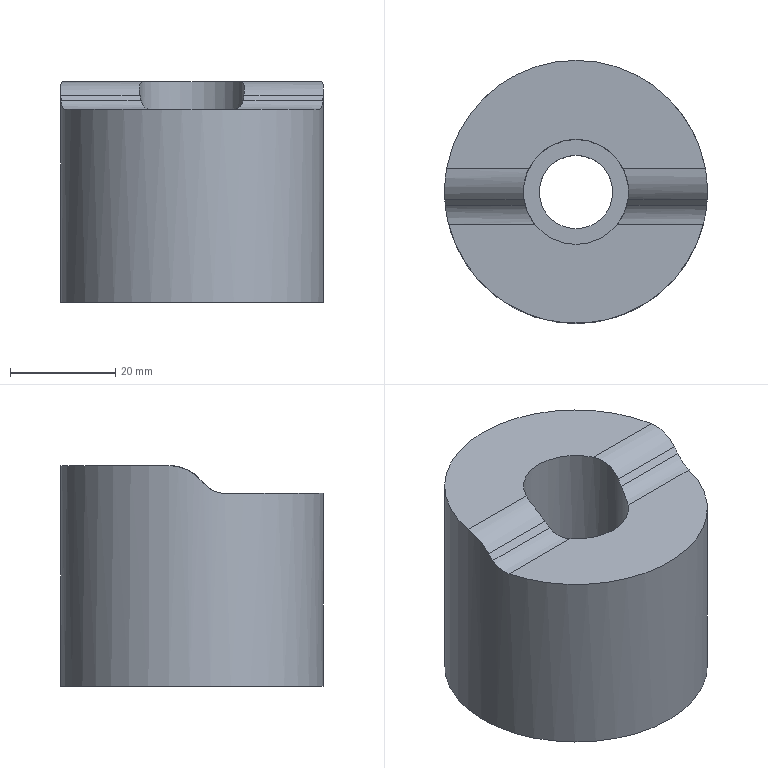Part | NX | features solid 2 | 1 solid | 13 faces | box 50 x 50 x 42.008 mm | volume 68340 mm3 | cylinder 7 | plane 6 | commonest cylinder face diameters 10 x2 16 x2 14 x1 20 x1 50 x1
STEP:
#1=CARTESIAN_POINT('',(215.,-615.,50.));
#2=VERTEX_POINT('',#1);
#3=CARTESIAN_POINT('',(215.,-590.,50.));
#4=DIRECTION('',(0.,0.,1.));
#5=DIRECTION('',(0.,-1.,0.));
#6=AXIS2_PLACEMENT_3D('',#3,#4,#5);
#7=CIRCLE('',#6,25.);
#8=EDGE_CURVE('',#2,#2,#7,.T.);
#9=ORIENTED_EDGE('',*,*,#8,.T.);
#10=EDGE_LOOP('',(#9));
#11=FACE_BOUND('',#10,.T.);
#12=CARTESIAN_POINT('',(239.954,-591.512,89.423));
#13=VERTEX_POINT('',#12);
#14=CARTESIAN_POINT('',(239.614,-585.624,92.008));
#15=VERTEX_POINT('',#14);
#16=CARTESIAN_POINT('',(239.954,-591.512,89.423));
#17=CARTESIAN_POINT('',(240.046,-590.003,91.064));
#18=CARTESIAN_POINT('',(240.005,-587.821,92.008));
#19=CARTESIAN_POINT('',(239.614,-585.624,92.008));
#20=B_SPLINE_CURVE_WITH_KNOTS('',3,(#16,#17,#18,#19),.UNSPECIFIED.,.F.,.F.,(4,4),(0.,0.006601),.UNSPECIFIED.);
#21=EDGE_CURVE('',#13,#15,#20,.T.);
#22=ORIENTED_EDGE('',*,*,#21,.F.);
#23=CARTESIAN_POINT('',(239.872,-592.524,88.323));
#24=VERTEX_POINT('',#23);
#25=CARTESIAN_POINT('',(215.,-590.,91.067));
#26=DIRECTION('',(0.,0.736,-0.677));
#27=DIRECTION('',(0.,-0.677,-0.736));
#28=AXIS2_PLACEMENT_3D('',#25,#26,#27);
#29=ELLIPSE('',#28,36.93,25.);
#30=EDGE_CURVE('',#13,#24,#29,.T.);
#31=ORIENTED_EDGE('',*,*,#30,.T.);
#32=CARTESIAN_POINT('',(239.218,-596.204,86.708));
#33=VERTEX_POINT('',#32);
#34=CARTESIAN_POINT('',(239.872,-592.524,88.323));
#35=CARTESIAN_POINT('',(239.776,-593.476,87.288));
#36=CARTESIAN_POINT('',(239.568,-594.839,86.708));
#37=CARTESIAN_POINT('',(239.218,-596.204,86.708));
#38=B_SPLINE_CURVE_WITH_KNOTS('',3,(#34,#35,#36,#37),.UNSPECIFIED.,.F.,.F.,(4,4),(0.,0.004167),.UNSPECIFIED.);
#39=EDGE_CURVE('',#24,#33,#38,.T.);
#40=ORIENTED_EDGE('',*,*,#39,.T.);
#41=CARTESIAN_POINT('',(190.782,-596.204,86.708));
#42=VERTEX_POINT('',#41);
#43=CARTESIAN_POINT('',(215.,-590.,86.708));
#44=DIRECTION('',(0.,0.,1.));
#45=DIRECTION('',(0.,-1.,0.));
#46=AXIS2_PLACEMENT_3D('',#43,#44,#45);
#47=CIRCLE('',#46,25.);
#48=EDGE_CURVE('',#42,#33,#47,.T.);
#49=ORIENTED_EDGE('',*,*,#48,.F.);
#50=CARTESIAN_POINT('',(190.128,-592.524,88.323));
#51=VERTEX_POINT('',#50);
#52=CARTESIAN_POINT('',(190.782,-596.204,86.708));
#53=CARTESIAN_POINT('',(190.432,-594.839,86.708));
#54=CARTESIAN_POINT('',(190.224,-593.476,87.288));
#55=CARTESIAN_POINT('',(190.128,-592.524,88.323));
#56=B_SPLINE_CURVE_WITH_KNOTS('',3,(#52,#53,#54,#55),.UNSPECIFIED.,.F.,.F.,(4,4),(0.,0.004169),.UNSPECIFIED.);
#57=EDGE_CURVE('',#42,#51,#56,.T.);
#58=ORIENTED_EDGE('',*,*,#57,.T.);
#59=CARTESIAN_POINT('',(190.046,-591.512,89.423));
#60=VERTEX_POINT('',#59);
#61=CARTESIAN_POINT('',(215.,-590.,91.067));
#62=DIRECTION('',(0.,0.736,-0.677));
#63=DIRECTION('',(0.,-0.677,-0.736));
#64=AXIS2_PLACEMENT_3D('',#61,#62,#63);
#65=ELLIPSE('',#64,36.93,25.);
#66=EDGE_CURVE('',#51,#60,#65,.T.);
#67=ORIENTED_EDGE('',*,*,#66,.T.);
#68=CARTESIAN_POINT('',(190.386,-585.624,92.008));
#69=VERTEX_POINT('',#68);
#70=CARTESIAN_POINT('',(190.386,-585.624,92.008));
#71=CARTESIAN_POINT('',(189.995,-587.821,92.008));
#72=CARTESIAN_POINT('',(189.954,-590.003,91.064));
#73=CARTESIAN_POINT('',(190.046,-591.512,89.423));
#74=B_SPLINE_CURVE_WITH_KNOTS('',3,(#70,#71,#72,#73),.UNSPECIFIED.,.F.,.F.,(4,4),(0.,0.006599),.UNSPECIFIED.);
#75=EDGE_CURVE('',#69,#60,#74,.T.);
#76=ORIENTED_EDGE('',*,*,#75,.F.);
#77=CARTESIAN_POINT('',(215.,-590.,92.008));
#78=DIRECTION('',(0.,0.,1.));
#79=DIRECTION('',(0.,-1.,0.));
#80=AXIS2_PLACEMENT_3D('',#77,#78,#79);
#81=CIRCLE('',#80,25.);
#82=EDGE_CURVE('',#15,#69,#81,.T.);
#83=ORIENTED_EDGE('',*,*,#82,.F.);
#84=EDGE_LOOP('',(#22,#31,#40,#49,#58,#67,#76,#83));
#85=FACE_BOUND('',#84,.T.);
#86=CARTESIAN_POINT('',(215.,-590.,100.));
#87=DIRECTION('',(0.,0.,-1.));
#88=DIRECTION('',(0.,1.,0.));
#89=AXIS2_PLACEMENT_3D('',#86,#87,#88);
#90=CYLINDRICAL_SURFACE('',#89,25.);
#91=ADVANCED_FACE('',(#11,#85),#90,.T.);
#92=CARTESIAN_POINT('',(215.,-597.,50.));
#93=VERTEX_POINT('',#92);
#94=CARTESIAN_POINT('',(215.,-590.,50.));
#95=DIRECTION('',(0.,0.,1.));
#96=DIRECTION('',(0.,-1.,0.));
#97=AXIS2_PLACEMENT_3D('',#94,#95,#96);
#98=CIRCLE('',#97,7.);
#99=EDGE_CURVE('',#93,#93,#98,.T.);
#100=ORIENTED_EDGE('',*,*,#99,.T.);
#101=EDGE_LOOP('',(#100));
#102=FACE_BOUND('',#101,.T.);
#103=ORIENTED_EDGE('',*,*,#8,.F.);
#104=EDGE_LOOP('',(#103));
#105=FACE_BOUND('',#104,.T.);
#106=CARTESIAN_POINT('',(215.,-590.,50.));
#107=DIRECTION('',(0.,0.,1.));
#108=DIRECTION('',(0.,-1.,0.));
#109=AXIS2_PLACEMENT_3D('',#106,#107,#108);
#110=PLANE('',#109);
#111=ADVANCED_FACE('',(#102,#105),#110,.F.);
#112=CARTESIAN_POINT('',(223.992,-585.624,92.008));
#113=VERTEX_POINT('',#112);
#114=CARTESIAN_POINT('',(223.992,-585.624,92.008));
#115=CARTESIAN_POINT('',(229.199,-585.624,92.008));
#116=CARTESIAN_POINT('',(234.407,-585.624,92.008));
#117=CARTESIAN_POINT('',(239.614,-585.624,92.008));
#118=B_SPLINE_CURVE_WITH_KNOTS('',3,(#114,#115,#116,#117),.UNSPECIFIED.,.F.,.F.,(4,4),(0.8313,0.8502),.UNSPECIFIED.);
#119=EDGE_CURVE('',#113,#15,#118,.T.);
#120=ORIENTED_EDGE('',*,*,#119,.T.);
#121=ORIENTED_EDGE('',*,*,#82,.T.);
#122=CARTESIAN_POINT('',(206.008,-585.624,92.008));
#123=VERTEX_POINT('',#122);
#124=CARTESIAN_POINT('',(190.386,-585.624,92.008));
#125=CARTESIAN_POINT('',(195.593,-585.624,92.008));
#126=CARTESIAN_POINT('',(200.801,-585.624,92.008));
#127=CARTESIAN_POINT('',(206.008,-585.624,92.008));
#128=B_SPLINE_CURVE_WITH_KNOTS('',3,(#124,#125,#126,#127),.UNSPECIFIED.,.F.,.F.,(4,4),(0.7907,0.8095),.UNSPECIFIED.);
#129=EDGE_CURVE('',#69,#123,#128,.T.);
#130=ORIENTED_EDGE('',*,*,#129,.T.);
#131=CARTESIAN_POINT('',(215.,-590.,92.008));
#132=DIRECTION('',(0.,0.,1.));
#133=DIRECTION('',(0.,-1.,0.));
#134=AXIS2_PLACEMENT_3D('',#131,#132,#133);
#135=CIRCLE('',#134,10.);
#136=EDGE_CURVE('',#123,#113,#135,.F.);
#137=ORIENTED_EDGE('',*,*,#136,.T.);
#138=EDGE_LOOP('',(#120,#121,#130,#137));
#139=FACE_BOUND('',#138,.T.);
#140=CARTESIAN_POINT('',(525.068,183.357,92.008));
#141=DIRECTION('',(0.,0.,1.));
#142=DIRECTION('',(0.,-1.,0.));
#143=AXIS2_PLACEMENT_3D('',#140,#141,#142);
#144=PLANE('',#143);
#145=ADVANCED_FACE('',(#139),#144,.T.);
#146=ORIENTED_EDGE('',*,*,#129,.F.);
#147=ORIENTED_EDGE('',*,*,#75,.T.);
#148=CARTESIAN_POINT('',(205.115,-591.512,89.423));
#149=VERTEX_POINT('',#148);
#150=CARTESIAN_POINT('',(190.046,-591.512,89.423));
#151=CARTESIAN_POINT('',(195.069,-591.512,89.423));
#152=CARTESIAN_POINT('',(200.092,-591.512,89.423));
#153=CARTESIAN_POINT('',(205.115,-591.512,89.423));
#154=B_SPLINE_CURVE_WITH_KNOTS('',3,(#150,#151,#152,#153),.UNSPECIFIED.,.F.,.F.,(4,4),(0.7903,0.8085),.UNSPECIFIED.);
#155=EDGE_CURVE('',#149,#60,#154,.F.);
#156=ORIENTED_EDGE('',*,*,#155,.F.);
#157=CARTESIAN_POINT('',(205.115,-591.512,89.423));
#158=CARTESIAN_POINT('',(204.998,-590.746,90.256));
#159=CARTESIAN_POINT('',(204.897,-588.853,91.59));
#160=CARTESIAN_POINT('',(205.51,-586.648,92.008));
#161=CARTESIAN_POINT('',(206.008,-585.624,92.008));
#162=B_SPLINE_CURVE_WITH_KNOTS('',3,(#157,#158,#159,#160,#161),.UNSPECIFIED.,.F.,.F.,(4,1,4),(0.,0.003371,0.006743),.UNSPECIFIED.);
#163=EDGE_CURVE('',#149,#123,#162,.T.);
#164=ORIENTED_EDGE('',*,*,#163,.T.);
#165=EDGE_LOOP('',(#146,#147,#156,#164));
#166=FACE_BOUND('',#165,.T.);
#167=CARTESIAN_POINT('',(6000363.634,-585.624,84.008));
#168=DIRECTION('',(-1.,0.,0.));
#169=DIRECTION('',(0.,0.,-1.));
#170=AXIS2_PLACEMENT_3D('',#167,#168,#169);
#171=CYLINDRICAL_SURFACE('',#170,8.);
#172=ADVANCED_FACE('',(#166),#171,.T.);
#173=CARTESIAN_POINT('',(224.885,-591.512,89.423));
#174=VERTEX_POINT('',#173);
#175=CARTESIAN_POINT('',(224.885,-591.512,89.423));
#176=CARTESIAN_POINT('',(229.908,-591.512,89.423));
#177=CARTESIAN_POINT('',(234.931,-591.512,89.423));
#178=CARTESIAN_POINT('',(239.954,-591.512,89.423));
#179=B_SPLINE_CURVE_WITH_KNOTS('',3,(#175,#176,#177,#178),.UNSPECIFIED.,.F.,.F.,(4,4),(0.8324,0.8506),.UNSPECIFIED.);
#180=EDGE_CURVE('',#13,#174,#179,.F.);
#181=ORIENTED_EDGE('',*,*,#180,.F.);
#182=ORIENTED_EDGE('',*,*,#21,.T.);
#183=ORIENTED_EDGE('',*,*,#119,.F.);
#184=CARTESIAN_POINT('',(223.992,-585.624,92.008));
#185=CARTESIAN_POINT('',(224.49,-586.648,92.008));
#186=CARTESIAN_POINT('',(225.103,-588.851,91.591));
#187=CARTESIAN_POINT('',(225.002,-590.746,90.256));
#188=CARTESIAN_POINT('',(224.885,-591.512,89.423));
#189=B_SPLINE_CURVE_WITH_KNOTS('',3,(#184,#185,#186,#187,#188),.UNSPECIFIED.,.F.,.F.,(4,1,4),(0.,0.00337,0.00674),.UNSPECIFIED.);
#190=EDGE_CURVE('',#113,#174,#189,.T.);
#191=ORIENTED_EDGE('',*,*,#190,.T.);
#192=EDGE_LOOP('',(#181,#182,#183,#191));
#193=FACE_BOUND('',#192,.T.);
#194=CARTESIAN_POINT('',(6000363.634,-585.624,84.008));
#195=DIRECTION('',(-1.,0.,0.));
#196=DIRECTION('',(0.,0.,-1.));
#197=AXIS2_PLACEMENT_3D('',#194,#195,#196);
#198=CYLINDRICAL_SURFACE('',#197,8.);
#199=ADVANCED_FACE('',(#193),#198,.T.);
#200=ORIENTED_EDGE('',*,*,#66,.F.);
#201=CARTESIAN_POINT('',(205.324,-592.524,88.323));
#202=VERTEX_POINT('',#201);
#203=CARTESIAN_POINT('',(205.324,-592.524,88.323));
#204=CARTESIAN_POINT('',(200.258,-592.524,88.323));
#205=CARTESIAN_POINT('',(195.193,-592.524,88.323));
#206=CARTESIAN_POINT('',(190.128,-592.524,88.323));
#207=B_SPLINE_CURVE_WITH_KNOTS('',3,(#203,#204,#205,#206),.UNSPECIFIED.,.F.,.F.,(4,4),(0.1913,0.2096),.UNSPECIFIED.);
#208=EDGE_CURVE('',#202,#51,#207,.T.);
#209=ORIENTED_EDGE('',*,*,#208,.F.);
#210=CARTESIAN_POINT('',(215.,-590.,91.067));
#211=DIRECTION('',(0.,0.736,-0.677));
#212=DIRECTION('',(0.,-0.677,-0.736));
#213=AXIS2_PLACEMENT_3D('',#210,#211,#212);
#214=ELLIPSE('',#213,14.772,10.);
#215=EDGE_CURVE('',#149,#202,#214,.F.);
#216=ORIENTED_EDGE('',*,*,#215,.F.);
#217=ORIENTED_EDGE('',*,*,#155,.T.);
#218=EDGE_LOOP('',(#200,#209,#216,#217));
#219=FACE_BOUND('',#218,.T.);
#220=CARTESIAN_POINT('',(-563.463,-663.442,11.217));
#221=DIRECTION('',(0.,0.736,-0.677));
#222=DIRECTION('',(0.,0.677,0.736));
#223=AXIS2_PLACEMENT_3D('',#220,#221,#222);
#224=PLANE('',#223);
#225=ADVANCED_FACE('',(#219),#224,.F.);
#226=ORIENTED_EDGE('',*,*,#30,.F.);
#227=ORIENTED_EDGE('',*,*,#180,.T.);
#228=CARTESIAN_POINT('',(224.676,-592.524,88.323));
#229=VERTEX_POINT('',#228);
#230=CARTESIAN_POINT('',(215.,-590.,91.067));
#231=DIRECTION('',(0.,0.736,-0.677));
#232=DIRECTION('',(0.,-0.677,-0.736));
#233=AXIS2_PLACEMENT_3D('',#230,#231,#232);
#234=ELLIPSE('',#233,14.772,10.);
#235=EDGE_CURVE('',#229,#174,#234,.F.);
#236=ORIENTED_EDGE('',*,*,#235,.F.);
#237=CARTESIAN_POINT('',(239.872,-592.524,88.323));
#238=CARTESIAN_POINT('',(234.807,-592.524,88.323));
#239=CARTESIAN_POINT('',(229.742,-592.524,88.323));
#240=CARTESIAN_POINT('',(224.676,-592.524,88.323));
#241=B_SPLINE_CURVE_WITH_KNOTS('',3,(#237,#238,#239,#240),.UNSPECIFIED.,.F.,.F.,(4,4),(0.1495,0.1679),.UNSPECIFIED.);
#242=EDGE_CURVE('',#24,#229,#241,.T.);
#243=ORIENTED_EDGE('',*,*,#242,.F.);
#244=EDGE_LOOP('',(#226,#227,#236,#243));
#245=FACE_BOUND('',#244,.T.);
#246=CARTESIAN_POINT('',(-563.463,-663.442,11.217));
#247=DIRECTION('',(0.,0.736,-0.677));
#248=DIRECTION('',(0.,0.677,0.736));
#249=AXIS2_PLACEMENT_3D('',#246,#247,#248);
#250=PLANE('',#249);
#251=ADVANCED_FACE('',(#245),#250,.F.);
#252=CARTESIAN_POINT('',(207.157,-596.204,86.708));
#253=VERTEX_POINT('',#252);
#254=CARTESIAN_POINT('',(207.157,-596.204,86.708));
#255=CARTESIAN_POINT('',(201.699,-596.204,86.708));
#256=CARTESIAN_POINT('',(196.24,-596.204,86.708));
#257=CARTESIAN_POINT('',(190.782,-596.204,86.708));
#258=B_SPLINE_CURVE_WITH_KNOTS('',3,(#254,#255,#256,#257),.UNSPECIFIED.,.F.,.F.,(4,4),(0.1891,0.2089),.UNSPECIFIED.);
#259=EDGE_CURVE('',#253,#42,#258,.T.);
#260=ORIENTED_EDGE('',*,*,#259,.T.);
#261=ORIENTED_EDGE('',*,*,#48,.T.);
#262=CARTESIAN_POINT('',(222.843,-596.204,86.708));
#263=VERTEX_POINT('',#262);
#264=CARTESIAN_POINT('',(239.218,-596.204,86.708));
#265=CARTESIAN_POINT('',(233.76,-596.204,86.708));
#266=CARTESIAN_POINT('',(228.301,-596.204,86.708));
#267=CARTESIAN_POINT('',(222.843,-596.204,86.708));
#268=B_SPLINE_CURVE_WITH_KNOTS('',3,(#264,#265,#266,#267),.UNSPECIFIED.,.F.,.F.,(4,4),(0.1503,0.1701),.UNSPECIFIED.);
#269=EDGE_CURVE('',#33,#263,#268,.T.);
#270=ORIENTED_EDGE('',*,*,#269,.T.);
#271=CARTESIAN_POINT('',(215.,-590.,86.708));
#272=DIRECTION('',(0.,0.,1.));
#273=DIRECTION('',(0.,-1.,0.));
#274=AXIS2_PLACEMENT_3D('',#271,#272,#273);
#275=CIRCLE('',#274,10.);
#276=EDGE_CURVE('',#263,#253,#275,.F.);
#277=ORIENTED_EDGE('',*,*,#276,.T.);
#278=EDGE_LOOP('',(#260,#261,#270,#277));
#279=FACE_BOUND('',#278,.T.);
#280=CARTESIAN_POINT('',(376.488,227.578,86.708));
#281=DIRECTION('',(0.,0.,1.));
#282=DIRECTION('',(0.,-1.,0.));
#283=AXIS2_PLACEMENT_3D('',#280,#281,#282);
#284=PLANE('',#283);
#285=ADVANCED_FACE('',(#279),#284,.T.);
#286=ORIENTED_EDGE('',*,*,#39,.F.);
#287=ORIENTED_EDGE('',*,*,#242,.T.);
#288=CARTESIAN_POINT('',(222.843,-596.204,86.708));
#289=CARTESIAN_POINT('',(223.795,-595.,86.708));
#290=CARTESIAN_POINT('',(224.408,-593.551,87.207));
#291=CARTESIAN_POINT('',(224.676,-592.524,88.323));
#292=B_SPLINE_CURVE_WITH_KNOTS('',3,(#288,#289,#290,#291),.UNSPECIFIED.,.F.,.F.,(4,4),(0.,0.00455),.UNSPECIFIED.);
#293=EDGE_CURVE('',#263,#229,#292,.T.);
#294=ORIENTED_EDGE('',*,*,#293,.F.);
#295=ORIENTED_EDGE('',*,*,#269,.F.);
#296=EDGE_LOOP('',(#286,#287,#294,#295));
#297=FACE_BOUND('',#296,.T.);
#298=CARTESIAN_POINT('',(-6000464.,-596.204,91.708));
#299=DIRECTION('',(1.,0.,0.));
#300=DIRECTION('',(0.,0.,1.));
#301=AXIS2_PLACEMENT_3D('',#298,#299,#300);
#302=CYLINDRICAL_SURFACE('',#301,5.);
#303=ADVANCED_FACE('',(#297),#302,.F.);
#304=ORIENTED_EDGE('',*,*,#57,.F.);
#305=ORIENTED_EDGE('',*,*,#259,.F.);
#306=CARTESIAN_POINT('',(205.324,-592.524,88.323));
#307=CARTESIAN_POINT('',(205.591,-593.549,87.208));
#308=CARTESIAN_POINT('',(206.205,-595.001,86.708));
#309=CARTESIAN_POINT('',(207.157,-596.204,86.708));
#310=B_SPLINE_CURVE_WITH_KNOTS('',3,(#306,#307,#308,#309),.UNSPECIFIED.,.F.,.F.,(4,4),(0.,0.004545),.UNSPECIFIED.);
#311=EDGE_CURVE('',#202,#253,#310,.T.);
#312=ORIENTED_EDGE('',*,*,#311,.F.);
#313=ORIENTED_EDGE('',*,*,#208,.T.);
#314=EDGE_LOOP('',(#304,#305,#312,#313));
#315=FACE_BOUND('',#314,.T.);
#316=CARTESIAN_POINT('',(-6000464.,-596.204,91.708));
#317=DIRECTION('',(1.,0.,0.));
#318=DIRECTION('',(0.,0.,1.));
#319=AXIS2_PLACEMENT_3D('',#316,#317,#318);
#320=CYLINDRICAL_SURFACE('',#319,5.);
#321=ADVANCED_FACE('',(#315),#320,.F.);
#322=CARTESIAN_POINT('',(215.,-583.,70.));
#323=VERTEX_POINT('',#322);
#324=CARTESIAN_POINT('',(215.,-590.,70.));
#325=DIRECTION('',(0.,0.,-1.));
#326=DIRECTION('',(0.,1.,0.));
#327=AXIS2_PLACEMENT_3D('',#324,#325,#326);
#328=CIRCLE('',#327,7.);
#329=EDGE_CURVE('',#323,#323,#328,.T.);
#330=ORIENTED_EDGE('',*,*,#329,.T.);
#331=EDGE_LOOP('',(#330));
#332=FACE_BOUND('',#331,.T.);
#333=CARTESIAN_POINT('',(215.,-580.,70.));
#334=VERTEX_POINT('',#333);
#335=CARTESIAN_POINT('',(215.,-590.,70.));
#336=DIRECTION('',(0.,0.,-1.));
#337=DIRECTION('',(0.,1.,0.));
#338=AXIS2_PLACEMENT_3D('',#335,#336,#337);
#339=CIRCLE('',#338,10.);
#340=EDGE_CURVE('',#334,#334,#339,.T.);
#341=ORIENTED_EDGE('',*,*,#340,.F.);
#342=EDGE_LOOP('',(#341));
#343=FACE_BOUND('',#342,.T.);
#344=CARTESIAN_POINT('',(215.,-590.,70.));
#345=DIRECTION('',(0.,0.,-1.));
#346=DIRECTION('',(0.,1.,0.));
#347=AXIS2_PLACEMENT_3D('',#344,#345,#346);
#348=PLANE('',#347);
#349=ADVANCED_FACE('',(#332,#343),#348,.F.);
#350=ORIENTED_EDGE('',*,*,#340,.T.);
#351=EDGE_LOOP('',(#350));
#352=FACE_BOUND('',#351,.T.);
#353=ORIENTED_EDGE('',*,*,#163,.F.);
#354=ORIENTED_EDGE('',*,*,#215,.T.);
#355=ORIENTED_EDGE('',*,*,#311,.T.);
#356=ORIENTED_EDGE('',*,*,#276,.F.);
#357=ORIENTED_EDGE('',*,*,#293,.T.);
#358=ORIENTED_EDGE('',*,*,#235,.T.);
#359=ORIENTED_EDGE('',*,*,#190,.F.);
#360=ORIENTED_EDGE('',*,*,#136,.F.);
#361=EDGE_LOOP('',(#353,#354,#355,#356,#357,#358,#359,#360));
#362=FACE_BOUND('',#361,.T.);
#363=CARTESIAN_POINT('',(215.,-590.,130.));
#364=DIRECTION('',(0.,0.,-1.));
#365=DIRECTION('',(0.,1.,0.));
#366=AXIS2_PLACEMENT_3D('',#363,#364,#365);
#367=CYLINDRICAL_SURFACE('',#366,10.);
#368=ADVANCED_FACE('',(#352,#362),#367,.F.);
#369=ORIENTED_EDGE('',*,*,#329,.F.);
#370=EDGE_LOOP('',(#369));
#371=FACE_BOUND('',#370,.T.);
#372=ORIENTED_EDGE('',*,*,#99,.F.);
#373=EDGE_LOOP('',(#372));
#374=FACE_BOUND('',#373,.T.);
#375=CARTESIAN_POINT('',(215.,-590.,70.));
#376=DIRECTION('',(0.,0.,-1.));
#377=DIRECTION('',(0.,1.,0.));
#378=AXIS2_PLACEMENT_3D('',#375,#376,#377);
#379=CYLINDRICAL_SURFACE('',#378,7.);
#380=ADVANCED_FACE('',(#371,#374),#379,.F.);
#381=CLOSED_SHELL('',(#91,#111,#145,#172,#199,#225,#251,#285,#303,#321,#349,#368,#380));
#382=MANIFOLD_SOLID_BREP('',#381);
#383=(LENGTH_UNIT()NAMED_UNIT(*)SI_UNIT(.MILLI.,.METRE.));
#384=UNCERTAINTY_MEASURE_WITH_UNIT(LENGTH_MEASURE(0.0508),#383,'','');
#385=(NAMED_UNIT(*)PLANE_ANGLE_UNIT()SI_UNIT($,.RADIAN.));
#386=(NAMED_UNIT(*)SI_UNIT($,.STERADIAN.)SOLID_ANGLE_UNIT());
#387=(GEOMETRIC_REPRESENTATION_CONTEXT(3)GLOBAL_UNCERTAINTY_ASSIGNED_CONTEXT((#384))GLOBAL_UNIT_ASSIGNED_CONTEXT((#383,#385,#386))REPRESENTATION_CONTEXT('',''));
#388=ADVANCED_BREP_SHAPE_REPRESENTATION('',(#382),#387);